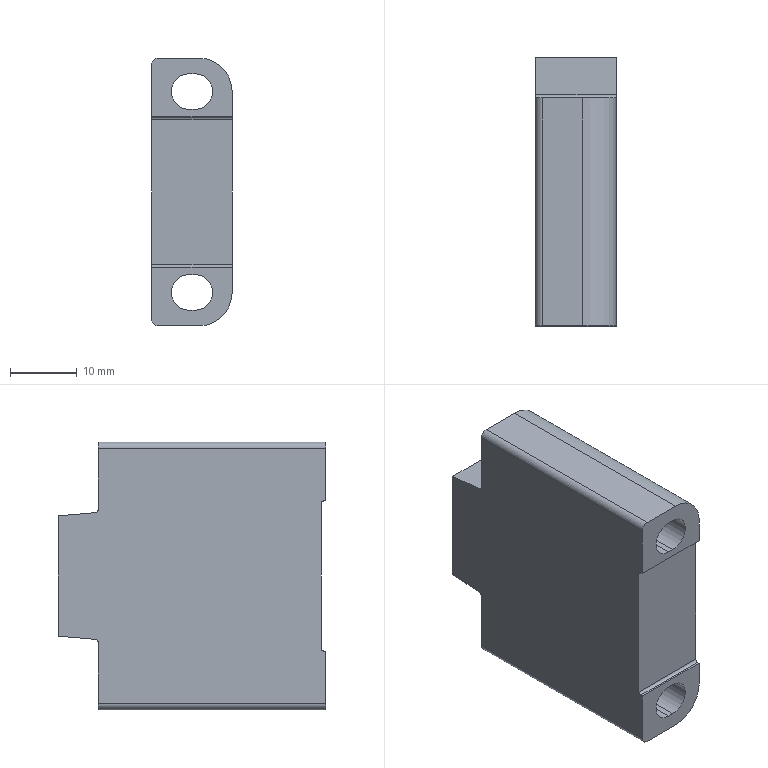Part | SolidWorks | features BaseBody 1 | 1 solid | 83 faces | box 12 x 40 x 40 mm | volume 13903 mm3 | plane 67 | cylinder 16 | commonest cylinder face diameters 5.3 x4 0.8 x2 1 x2 2 x2 5 x2 10 x2